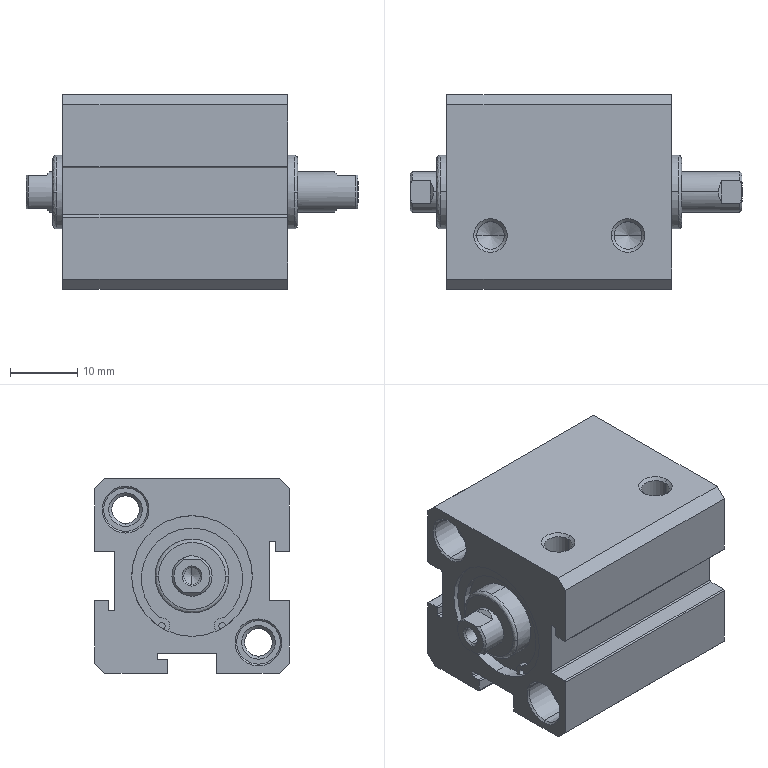Part | SolidWorks | 2 solids | 205 faces | box 49.5 x 29 x 29 mm | volume 22629 mm3 | cylinder 89 | plane 61 | cone 43 | spline 12 | commonest cylinder face diameters 0.4 x18 1 x12 4.134 x8 6 x8 6.5 x8 2.4 x6